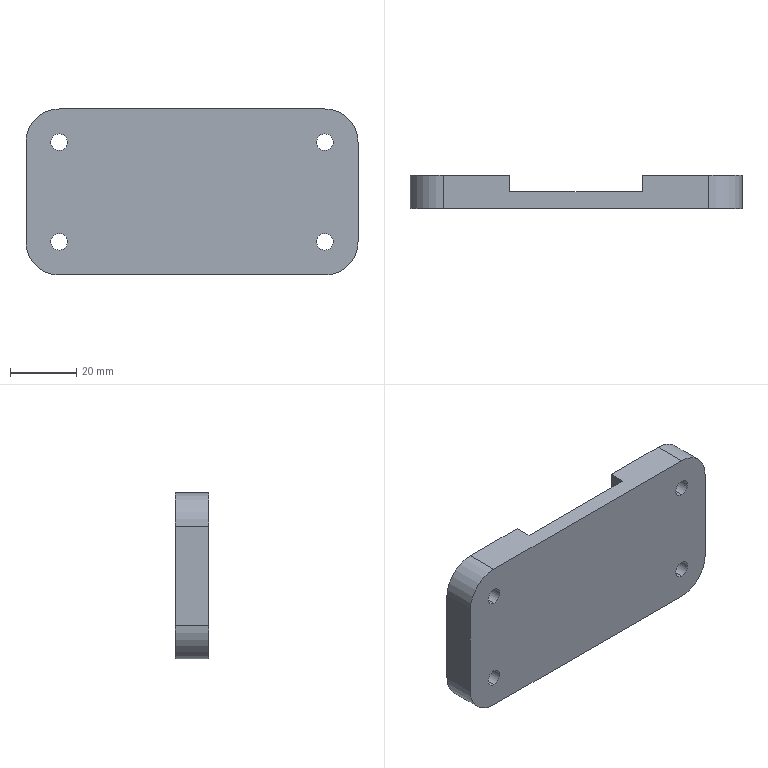Part | SolidWorks | features 3DProfileFeature 1, Extrusion 1, Fillet 1, HoleWzd 1, ICE 1 | 1 solid | 22 faces | box 100 x 10 x 50 mm | volume 38356 mm3 | cylinder 12 | plane 10 | commonest cylinder face diameters 5 x8 20 x4
STEP:
#1=CARTESIAN_POINT('',(-40.,0.,17.5));
#2=VERTEX_POINT('',#1);
#3=CARTESIAN_POINT('',(-40.,0.,12.5));
#4=VERTEX_POINT('',#3);
#5=CARTESIAN_POINT('',(-40.,0.,15.));
#6=DIRECTION('',(0.,-1.,0.));
#7=DIRECTION('',(0.,0.,-1.));
#8=AXIS2_PLACEMENT_3D('',#5,#6,#7);
#9=CIRCLE('',#8,2.5);
#10=EDGE_CURVE('',#2,#4,#9,.T.);
#11=ORIENTED_EDGE('',*,*,#10,.T.);
#12=CARTESIAN_POINT('',(-40.,10.,12.5));
#13=VERTEX_POINT('',#12);
#14=CARTESIAN_POINT('',(-40.,10.,12.5));
#15=DIRECTION('',(0.,1.,0.));
#16=VECTOR('',#15,1000.);
#17=LINE('',#14,#16);
#18=EDGE_CURVE('',#4,#13,#17,.T.);
#19=ORIENTED_EDGE('',*,*,#18,.T.);
#20=CARTESIAN_POINT('',(-40.,10.,17.5));
#21=VERTEX_POINT('',#20);
#22=CARTESIAN_POINT('',(-40.,10.,15.));
#23=DIRECTION('',(0.,1.,0.));
#24=DIRECTION('',(0.,0.,1.));
#25=AXIS2_PLACEMENT_3D('',#22,#23,#24);
#26=CIRCLE('',#25,2.5);
#27=EDGE_CURVE('',#13,#21,#26,.T.);
#28=ORIENTED_EDGE('',*,*,#27,.T.);
#29=CARTESIAN_POINT('',(-40.,10.,17.5));
#30=DIRECTION('',(0.,1.,0.));
#31=VECTOR('',#30,1000.);
#32=LINE('',#29,#31);
#33=EDGE_CURVE('',#2,#21,#32,.T.);
#34=ORIENTED_EDGE('',*,*,#33,.F.);
#35=EDGE_LOOP('',(#11,#19,#28,#34));
#36=FACE_OUTER_BOUND('',#35,.T.);
#37=CARTESIAN_POINT('',(-40.,10.,15.));
#38=DIRECTION('',(0.,1.,0.));
#39=DIRECTION('',(0.,0.,1.));
#40=AXIS2_PLACEMENT_3D('',#37,#38,#39);
#41=CYLINDRICAL_SURFACE('',#40,2.5);
#42=ADVANCED_FACE('',(#36),#41,.F.);
#43=CARTESIAN_POINT('',(-40.,0.,-12.5));
#44=VERTEX_POINT('',#43);
#45=CARTESIAN_POINT('',(-40.,0.,-17.5));
#46=VERTEX_POINT('',#45);
#47=CARTESIAN_POINT('',(-40.,0.,-15.));
#48=DIRECTION('',(0.,-1.,0.));
#49=DIRECTION('',(0.,0.,-1.));
#50=AXIS2_PLACEMENT_3D('',#47,#48,#49);
#51=CIRCLE('',#50,2.5);
#52=EDGE_CURVE('',#44,#46,#51,.T.);
#53=ORIENTED_EDGE('',*,*,#52,.T.);
#54=CARTESIAN_POINT('',(-40.,10.,-17.5));
#55=VERTEX_POINT('',#54);
#56=CARTESIAN_POINT('',(-40.,10.,-17.5));
#57=DIRECTION('',(0.,1.,0.));
#58=VECTOR('',#57,1000.);
#59=LINE('',#56,#58);
#60=EDGE_CURVE('',#46,#55,#59,.T.);
#61=ORIENTED_EDGE('',*,*,#60,.T.);
#62=CARTESIAN_POINT('',(-40.,10.,-12.5));
#63=VERTEX_POINT('',#62);
#64=CARTESIAN_POINT('',(-40.,10.,-15.));
#65=DIRECTION('',(0.,1.,0.));
#66=DIRECTION('',(0.,0.,1.));
#67=AXIS2_PLACEMENT_3D('',#64,#65,#66);
#68=CIRCLE('',#67,2.5);
#69=EDGE_CURVE('',#55,#63,#68,.T.);
#70=ORIENTED_EDGE('',*,*,#69,.T.);
#71=CARTESIAN_POINT('',(-40.,10.,-12.5));
#72=DIRECTION('',(0.,1.,0.));
#73=VECTOR('',#72,1000.);
#74=LINE('',#71,#73);
#75=EDGE_CURVE('',#44,#63,#74,.T.);
#76=ORIENTED_EDGE('',*,*,#75,.F.);
#77=EDGE_LOOP('',(#53,#61,#70,#76));
#78=FACE_OUTER_BOUND('',#77,.T.);
#79=CARTESIAN_POINT('',(-40.,10.,-15.));
#80=DIRECTION('',(0.,1.,0.));
#81=DIRECTION('',(0.,0.,1.));
#82=AXIS2_PLACEMENT_3D('',#79,#80,#81);
#83=CYLINDRICAL_SURFACE('',#82,2.5);
#84=ADVANCED_FACE('',(#78),#83,.F.);
#85=CARTESIAN_POINT('',(40.,0.,-12.5));
#86=VERTEX_POINT('',#85);
#87=CARTESIAN_POINT('',(40.,0.,-17.5));
#88=VERTEX_POINT('',#87);
#89=CARTESIAN_POINT('',(40.,0.,-15.));
#90=DIRECTION('',(0.,-1.,0.));
#91=DIRECTION('',(0.,0.,-1.));
#92=AXIS2_PLACEMENT_3D('',#89,#90,#91);
#93=CIRCLE('',#92,2.5);
#94=EDGE_CURVE('',#86,#88,#93,.T.);
#95=ORIENTED_EDGE('',*,*,#94,.T.);
#96=CARTESIAN_POINT('',(40.,10.,-17.5));
#97=VERTEX_POINT('',#96);
#98=CARTESIAN_POINT('',(40.,10.,-17.5));
#99=DIRECTION('',(0.,1.,0.));
#100=VECTOR('',#99,1000.);
#101=LINE('',#98,#100);
#102=EDGE_CURVE('',#88,#97,#101,.T.);
#103=ORIENTED_EDGE('',*,*,#102,.T.);
#104=CARTESIAN_POINT('',(40.,10.,-12.5));
#105=VERTEX_POINT('',#104);
#106=CARTESIAN_POINT('',(40.,10.,-15.));
#107=DIRECTION('',(0.,1.,0.));
#108=DIRECTION('',(0.,0.,1.));
#109=AXIS2_PLACEMENT_3D('',#106,#107,#108);
#110=CIRCLE('',#109,2.5);
#111=EDGE_CURVE('',#97,#105,#110,.T.);
#112=ORIENTED_EDGE('',*,*,#111,.T.);
#113=CARTESIAN_POINT('',(40.,10.,-12.5));
#114=DIRECTION('',(0.,1.,0.));
#115=VECTOR('',#114,1000.);
#116=LINE('',#113,#115);
#117=EDGE_CURVE('',#86,#105,#116,.T.);
#118=ORIENTED_EDGE('',*,*,#117,.F.);
#119=EDGE_LOOP('',(#95,#103,#112,#118));
#120=FACE_OUTER_BOUND('',#119,.T.);
#121=CARTESIAN_POINT('',(40.,10.,-15.));
#122=DIRECTION('',(0.,1.,0.));
#123=DIRECTION('',(0.,0.,1.));
#124=AXIS2_PLACEMENT_3D('',#121,#122,#123);
#125=CYLINDRICAL_SURFACE('',#124,2.5);
#126=ADVANCED_FACE('',(#120),#125,.F.);
#127=CARTESIAN_POINT('',(40.,0.,17.5));
#128=VERTEX_POINT('',#127);
#129=CARTESIAN_POINT('',(40.,0.,12.5));
#130=VERTEX_POINT('',#129);
#131=CARTESIAN_POINT('',(40.,0.,15.));
#132=DIRECTION('',(0.,-1.,0.));
#133=DIRECTION('',(0.,0.,-1.));
#134=AXIS2_PLACEMENT_3D('',#131,#132,#133);
#135=CIRCLE('',#134,2.5);
#136=EDGE_CURVE('',#128,#130,#135,.T.);
#137=ORIENTED_EDGE('',*,*,#136,.T.);
#138=CARTESIAN_POINT('',(40.,10.,12.5));
#139=VERTEX_POINT('',#138);
#140=CARTESIAN_POINT('',(40.,10.,12.5));
#141=DIRECTION('',(0.,1.,0.));
#142=VECTOR('',#141,1000.);
#143=LINE('',#140,#142);
#144=EDGE_CURVE('',#130,#139,#143,.T.);
#145=ORIENTED_EDGE('',*,*,#144,.T.);
#146=CARTESIAN_POINT('',(40.,10.,17.5));
#147=VERTEX_POINT('',#146);
#148=CARTESIAN_POINT('',(40.,10.,15.));
#149=DIRECTION('',(0.,1.,0.));
#150=DIRECTION('',(0.,0.,1.));
#151=AXIS2_PLACEMENT_3D('',#148,#149,#150);
#152=CIRCLE('',#151,2.5);
#153=EDGE_CURVE('',#139,#147,#152,.T.);
#154=ORIENTED_EDGE('',*,*,#153,.T.);
#155=CARTESIAN_POINT('',(40.,10.,17.5));
#156=DIRECTION('',(0.,1.,0.));
#157=VECTOR('',#156,1000.);
#158=LINE('',#155,#157);
#159=EDGE_CURVE('',#128,#147,#158,.T.);
#160=ORIENTED_EDGE('',*,*,#159,.F.);
#161=EDGE_LOOP('',(#137,#145,#154,#160));
#162=FACE_OUTER_BOUND('',#161,.T.);
#163=CARTESIAN_POINT('',(40.,10.,15.));
#164=DIRECTION('',(0.,1.,0.));
#165=DIRECTION('',(0.,0.,1.));
#166=AXIS2_PLACEMENT_3D('',#163,#164,#165);
#167=CYLINDRICAL_SURFACE('',#166,2.5);
#168=ADVANCED_FACE('',(#162),#167,.F.);
#169=CARTESIAN_POINT('',(40.,10.,15.));
#170=DIRECTION('',(0.,1.,0.));
#171=DIRECTION('',(0.,0.,1.));
#172=AXIS2_PLACEMENT_3D('',#169,#170,#171);
#173=CIRCLE('',#172,2.5);
#174=EDGE_CURVE('',#147,#139,#173,.T.);
#175=ORIENTED_EDGE('',*,*,#174,.F.);
#176=ORIENTED_EDGE('',*,*,#153,.F.);
#177=EDGE_LOOP('',(#175,#176));
#178=FACE_BOUND('',#177,.T.);
#179=CARTESIAN_POINT('',(40.,10.,-15.));
#180=DIRECTION('',(0.,1.,0.));
#181=DIRECTION('',(0.,0.,1.));
#182=AXIS2_PLACEMENT_3D('',#179,#180,#181);
#183=CIRCLE('',#182,2.5);
#184=EDGE_CURVE('',#105,#97,#183,.T.);
#185=ORIENTED_EDGE('',*,*,#184,.F.);
#186=ORIENTED_EDGE('',*,*,#111,.F.);
#187=EDGE_LOOP('',(#185,#186));
#188=FACE_BOUND('',#187,.T.);
#189=CARTESIAN_POINT('',(40.,10.,-25.));
#190=VERTEX_POINT('',#189);
#191=CARTESIAN_POINT('',(20.,10.,-25.));
#192=VERTEX_POINT('',#191);
#193=CARTESIAN_POINT('',(-50.,10.,-25.));
#194=DIRECTION('',(-1.,0.,0.));
#195=VECTOR('',#194,1000.);
#196=LINE('',#193,#195);
#197=EDGE_CURVE('',#190,#192,#196,.T.);
#198=ORIENTED_EDGE('',*,*,#197,.T.);
#199=CARTESIAN_POINT('',(20.,10.,25.));
#200=VERTEX_POINT('',#199);
#201=CARTESIAN_POINT('',(20.,10.,25.));
#202=DIRECTION('',(0.,0.,-1.));
#203=VECTOR('',#202,1000.);
#204=LINE('',#201,#203);
#205=EDGE_CURVE('',#200,#192,#204,.T.);
#206=ORIENTED_EDGE('',*,*,#205,.F.);
#207=CARTESIAN_POINT('',(40.,10.,25.));
#208=VERTEX_POINT('',#207);
#209=CARTESIAN_POINT('',(-50.,10.,25.));
#210=DIRECTION('',(1.,0.,0.));
#211=VECTOR('',#210,1000.);
#212=LINE('',#209,#211);
#213=EDGE_CURVE('',#200,#208,#212,.T.);
#214=ORIENTED_EDGE('',*,*,#213,.T.);
#215=CARTESIAN_POINT('',(50.,10.,15.));
#216=VERTEX_POINT('',#215);
#217=CARTESIAN_POINT('',(40.,10.,15.));
#218=DIRECTION('',(0.,1.,0.));
#219=DIRECTION('',(0.,0.,-1.));
#220=AXIS2_PLACEMENT_3D('',#217,#218,#219);
#221=CIRCLE('',#220,10.);
#222=EDGE_CURVE('',#208,#216,#221,.T.);
#223=ORIENTED_EDGE('',*,*,#222,.T.);
#224=CARTESIAN_POINT('',(50.,10.,-15.));
#225=VERTEX_POINT('',#224);
#226=CARTESIAN_POINT('',(50.,10.,25.));
#227=DIRECTION('',(0.,0.,-1.));
#228=VECTOR('',#227,1000.);
#229=LINE('',#226,#228);
#230=EDGE_CURVE('',#216,#225,#229,.T.);
#231=ORIENTED_EDGE('',*,*,#230,.T.);
#232=CARTESIAN_POINT('',(40.,10.,-15.));
#233=DIRECTION('',(0.,1.,0.));
#234=DIRECTION('',(0.,0.,-1.));
#235=AXIS2_PLACEMENT_3D('',#232,#233,#234);
#236=CIRCLE('',#235,10.);
#237=EDGE_CURVE('',#225,#190,#236,.T.);
#238=ORIENTED_EDGE('',*,*,#237,.T.);
#239=EDGE_LOOP('',(#198,#206,#214,#223,#231,#238));
#240=FACE_OUTER_BOUND('',#239,.T.);
#241=CARTESIAN_POINT('',(0.,10.,0.));
#242=DIRECTION('',(0.,-1.,0.));
#243=DIRECTION('',(0.,0.,-1.));
#244=AXIS2_PLACEMENT_3D('',#241,#242,#243);
#245=PLANE('',#244);
#246=ADVANCED_FACE('',(#178,#188,#240),#245,.F.);
#247=CARTESIAN_POINT('',(50.,0.,15.));
#248=VERTEX_POINT('',#247);
#249=CARTESIAN_POINT('',(50.,0.,-15.));
#250=VERTEX_POINT('',#249);
#251=CARTESIAN_POINT('',(50.,0.,25.));
#252=DIRECTION('',(0.,0.,-1.));
#253=VECTOR('',#252,1000.);
#254=LINE('',#251,#253);
#255=EDGE_CURVE('',#248,#250,#254,.T.);
#256=ORIENTED_EDGE('',*,*,#255,.T.);
#257=CARTESIAN_POINT('',(50.,10.,-15.));
#258=DIRECTION('',(0.,1.,0.));
#259=VECTOR('',#258,1000.);
#260=LINE('',#257,#259);
#261=EDGE_CURVE('',#250,#225,#260,.T.);
#262=ORIENTED_EDGE('',*,*,#261,.T.);
#263=ORIENTED_EDGE('',*,*,#230,.F.);
#264=CARTESIAN_POINT('',(50.,10.,15.));
#265=DIRECTION('',(0.,-1.,0.));
#266=VECTOR('',#265,1000.);
#267=LINE('',#264,#266);
#268=EDGE_CURVE('',#216,#248,#267,.T.);
#269=ORIENTED_EDGE('',*,*,#268,.T.);
#270=EDGE_LOOP('',(#256,#262,#263,#269));
#271=FACE_OUTER_BOUND('',#270,.T.);
#272=CARTESIAN_POINT('',(50.,10.,25.));
#273=DIRECTION('',(-1.,0.,0.));
#274=DIRECTION('',(0.,0.,1.));
#275=AXIS2_PLACEMENT_3D('',#272,#273,#274);
#276=PLANE('',#275);
#277=ADVANCED_FACE('',(#271),#276,.F.);
#278=CARTESIAN_POINT('',(20.,5.,-25.));
#279=VERTEX_POINT('',#278);
#280=CARTESIAN_POINT('',(-20.,5.,-25.));
#281=VERTEX_POINT('',#280);
#282=CARTESIAN_POINT('',(-20.,5.,-25.));
#283=DIRECTION('',(-1.,0.,0.));
#284=VECTOR('',#283,1000.);
#285=LINE('',#282,#284);
#286=EDGE_CURVE('',#279,#281,#285,.T.);
#287=ORIENTED_EDGE('',*,*,#286,.F.);
#288=CARTESIAN_POINT('',(20.,5.,-25.));
#289=DIRECTION('',(0.,1.,0.));
#290=VECTOR('',#289,1000.);
#291=LINE('',#288,#290);
#292=EDGE_CURVE('',#279,#192,#291,.T.);
#293=ORIENTED_EDGE('',*,*,#292,.T.);
#294=ORIENTED_EDGE('',*,*,#197,.F.);
#295=CARTESIAN_POINT('',(40.,0.,-25.));
#296=VERTEX_POINT('',#295);
#297=CARTESIAN_POINT('',(40.,10.,-25.));
#298=DIRECTION('',(0.,-1.,0.));
#299=VECTOR('',#298,1000.);
#300=LINE('',#297,#299);
#301=EDGE_CURVE('',#190,#296,#300,.T.);
#302=ORIENTED_EDGE('',*,*,#301,.T.);
#303=CARTESIAN_POINT('',(-40.,0.,-25.));
#304=VERTEX_POINT('',#303);
#305=CARTESIAN_POINT('',(-50.,0.,-25.));
#306=DIRECTION('',(-1.,0.,0.));
#307=VECTOR('',#306,1000.);
#308=LINE('',#305,#307);
#309=EDGE_CURVE('',#296,#304,#308,.T.);
#310=ORIENTED_EDGE('',*,*,#309,.T.);
#311=CARTESIAN_POINT('',(-40.,10.,-25.));
#312=VERTEX_POINT('',#311);
#313=CARTESIAN_POINT('',(-40.,10.,-25.));
#314=DIRECTION('',(0.,1.,0.));
#315=VECTOR('',#314,1000.);
#316=LINE('',#313,#315);
#317=EDGE_CURVE('',#304,#312,#316,.T.);
#318=ORIENTED_EDGE('',*,*,#317,.T.);
#319=CARTESIAN_POINT('',(-20.,10.,-25.));
#320=VERTEX_POINT('',#319);
#321=CARTESIAN_POINT('',(-50.,10.,-25.));
#322=DIRECTION('',(-1.,0.,0.));
#323=VECTOR('',#322,1000.);
#324=LINE('',#321,#323);
#325=EDGE_CURVE('',#320,#312,#324,.T.);
#326=ORIENTED_EDGE('',*,*,#325,.F.);
#327=CARTESIAN_POINT('',(-20.,5.,-25.));
#328=DIRECTION('',(0.,1.,0.));
#329=VECTOR('',#328,1000.);
#330=LINE('',#327,#329);
#331=EDGE_CURVE('',#281,#320,#330,.T.);
#332=ORIENTED_EDGE('',*,*,#331,.F.);
#333=EDGE_LOOP('',(#287,#293,#294,#302,#310,#318,#326,#332));
#334=FACE_OUTER_BOUND('',#333,.T.);
#335=CARTESIAN_POINT('',(-50.,10.,-25.));
#336=DIRECTION('',(0.,0.,1.));
#337=DIRECTION('',(1.,0.,0.));
#338=AXIS2_PLACEMENT_3D('',#335,#336,#337);
#339=PLANE('',#338);
#340=ADVANCED_FACE('',(#334),#339,.F.);
#341=CARTESIAN_POINT('',(-50.,10.,-15.));
#342=VERTEX_POINT('',#341);
#343=CARTESIAN_POINT('',(-50.,10.,15.));
#344=VERTEX_POINT('',#343);
#345=CARTESIAN_POINT('',(-50.,10.,25.));
#346=DIRECTION('',(0.,0.,1.));
#347=VECTOR('',#346,1000.);
#348=LINE('',#345,#347);
#349=EDGE_CURVE('',#342,#344,#348,.T.);
#350=ORIENTED_EDGE('',*,*,#349,.F.);
#351=CARTESIAN_POINT('',(-50.,0.,-15.));
#352=VERTEX_POINT('',#351);
#353=CARTESIAN_POINT('',(-50.,10.,-15.));
#354=DIRECTION('',(0.,-1.,0.));
#355=VECTOR('',#354,1000.);
#356=LINE('',#353,#355);
#357=EDGE_CURVE('',#342,#352,#356,.T.);
#358=ORIENTED_EDGE('',*,*,#357,.T.);
#359=CARTESIAN_POINT('',(-50.,0.,15.));
#360=VERTEX_POINT('',#359);
#361=CARTESIAN_POINT('',(-50.,0.,25.));
#362=DIRECTION('',(0.,0.,1.));
#363=VECTOR('',#362,1000.);
#364=LINE('',#361,#363);
#365=EDGE_CURVE('',#352,#360,#364,.T.);
#366=ORIENTED_EDGE('',*,*,#365,.T.);
#367=CARTESIAN_POINT('',(-50.,10.,15.));
#368=DIRECTION('',(0.,1.,0.));
#369=VECTOR('',#368,1000.);
#370=LINE('',#367,#369);
#371=EDGE_CURVE('',#360,#344,#370,.T.);
#372=ORIENTED_EDGE('',*,*,#371,.T.);
#373=EDGE_LOOP('',(#350,#358,#366,#372));
#374=FACE_OUTER_BOUND('',#373,.T.);
#375=CARTESIAN_POINT('',(-50.,10.,25.));
#376=DIRECTION('',(1.,0.,0.));
#377=DIRECTION('',(0.,0.,-1.));
#378=AXIS2_PLACEMENT_3D('',#375,#376,#377);
#379=PLANE('',#378);
#380=ADVANCED_FACE('',(#374),#379,.F.);
#381=ORIENTED_EDGE('',*,*,#213,.F.);
#382=CARTESIAN_POINT('',(20.,5.,25.));
#383=VERTEX_POINT('',#382);
#384=CARTESIAN_POINT('',(20.,5.,25.));
#385=DIRECTION('',(0.,1.,0.));
#386=VECTOR('',#385,1000.);
#387=LINE('',#384,#386);
#388=EDGE_CURVE('',#383,#200,#387,.T.);
#389=ORIENTED_EDGE('',*,*,#388,.F.);
#390=CARTESIAN_POINT('',(-20.,5.,25.));
#391=VERTEX_POINT('',#390);
#392=CARTESIAN_POINT('',(-20.,5.,25.));
#393=DIRECTION('',(1.,0.,0.));
#394=VECTOR('',#393,1000.);
#395=LINE('',#392,#394);
#396=EDGE_CURVE('',#391,#383,#395,.T.);
#397=ORIENTED_EDGE('',*,*,#396,.F.);
#398=CARTESIAN_POINT('',(-20.,10.,25.));
#399=VERTEX_POINT('',#398);
#400=CARTESIAN_POINT('',(-20.,5.,25.));
#401=DIRECTION('',(0.,1.,0.));
#402=VECTOR('',#401,1000.);
#403=LINE('',#400,#402);
#404=EDGE_CURVE('',#391,#399,#403,.T.);
#405=ORIENTED_EDGE('',*,*,#404,.T.);
#406=CARTESIAN_POINT('',(-40.,10.,25.));
#407=VERTEX_POINT('',#406);
#408=CARTESIAN_POINT('',(-50.,10.,25.));
#409=DIRECTION('',(1.,0.,0.));
#410=VECTOR('',#409,1000.);
#411=LINE('',#408,#410);
#412=EDGE_CURVE('',#407,#399,#411,.T.);
#413=ORIENTED_EDGE('',*,*,#412,.F.);
#414=CARTESIAN_POINT('',(-40.,0.,25.));
#415=VERTEX_POINT('',#414);
#416=CARTESIAN_POINT('',(-40.,10.,25.));
#417=DIRECTION('',(0.,-1.,0.));
#418=VECTOR('',#417,1000.);
#419=LINE('',#416,#418);
#420=EDGE_CURVE('',#407,#415,#419,.T.);
#421=ORIENTED_EDGE('',*,*,#420,.T.);
#422=CARTESIAN_POINT('',(40.,0.,25.));
#423=VERTEX_POINT('',#422);
#424=CARTESIAN_POINT('',(-50.,0.,25.));
#425=DIRECTION('',(1.,0.,0.));
#426=VECTOR('',#425,1000.);
#427=LINE('',#424,#426);
#428=EDGE_CURVE('',#415,#423,#427,.T.);
#429=ORIENTED_EDGE('',*,*,#428,.T.);
#430=CARTESIAN_POINT('',(40.,10.,25.));
#431=DIRECTION('',(0.,1.,0.));
#432=VECTOR('',#431,1000.);
#433=LINE('',#430,#432);
#434=EDGE_CURVE('',#423,#208,#433,.T.);
#435=ORIENTED_EDGE('',*,*,#434,.T.);
#436=EDGE_LOOP('',(#381,#389,#397,#405,#413,#421,#429,#435));
#437=FACE_OUTER_BOUND('',#436,.T.);
#438=CARTESIAN_POINT('',(-50.,10.,25.));
#439=DIRECTION('',(0.,0.,-1.));
#440=DIRECTION('',(-1.,0.,0.));
#441=AXIS2_PLACEMENT_3D('',#438,#439,#440);
#442=PLANE('',#441);
#443=ADVANCED_FACE('',(#437),#442,.F.);
#444=CARTESIAN_POINT('',(-40.,10.,15.));
#445=DIRECTION('',(0.,1.,0.));
#446=DIRECTION('',(0.,0.,1.));
#447=AXIS2_PLACEMENT_3D('',#444,#445,#446);
#448=CIRCLE('',#447,2.5);
#449=EDGE_CURVE('',#21,#13,#448,.T.);
#450=ORIENTED_EDGE('',*,*,#449,.F.);
#451=ORIENTED_EDGE('',*,*,#27,.F.);
#452=EDGE_LOOP('',(#450,#451));
#453=FACE_BOUND('',#452,.T.);
#454=CARTESIAN_POINT('',(-40.,10.,-15.));
#455=DIRECTION('',(0.,1.,0.));
#456=DIRECTION('',(0.,0.,1.));
#457=AXIS2_PLACEMENT_3D('',#454,#455,#456);
#458=CIRCLE('',#457,2.5);
#459=EDGE_CURVE('',#63,#55,#458,.T.);
#460=ORIENTED_EDGE('',*,*,#459,.F.);
#461=ORIENTED_EDGE('',*,*,#69,.F.);
#462=EDGE_LOOP('',(#460,#461));
#463=FACE_BOUND('',#462,.T.);
#464=ORIENTED_EDGE('',*,*,#412,.T.);
#465=CARTESIAN_POINT('',(-20.,10.,25.));
#466=DIRECTION('',(0.,0.,1.));
#467=VECTOR('',#466,1000.);
#468=LINE('',#465,#467);
#469=EDGE_CURVE('',#320,#399,#468,.T.);
#470=ORIENTED_EDGE('',*,*,#469,.F.);
#471=ORIENTED_EDGE('',*,*,#325,.T.);
#472=CARTESIAN_POINT('',(-40.,10.,-15.));
#473=DIRECTION('',(0.,1.,0.));
#474=DIRECTION('',(0.,0.,-1.));
#475=AXIS2_PLACEMENT_3D('',#472,#473,#474);
#476=CIRCLE('',#475,10.);
#477=EDGE_CURVE('',#312,#342,#476,.T.);
#478=ORIENTED_EDGE('',*,*,#477,.T.);
#479=ORIENTED_EDGE('',*,*,#349,.T.);
#480=CARTESIAN_POINT('',(-40.,10.,15.));
#481=DIRECTION('',(0.,1.,0.));
#482=DIRECTION('',(0.,0.,-1.));
#483=AXIS2_PLACEMENT_3D('',#480,#481,#482);
#484=CIRCLE('',#483,10.);
#485=EDGE_CURVE('',#344,#407,#484,.T.);
#486=ORIENTED_EDGE('',*,*,#485,.T.);
#487=EDGE_LOOP('',(#464,#470,#471,#478,#479,#486));
#488=FACE_OUTER_BOUND('',#487,.T.);
#489=CARTESIAN_POINT('',(0.,10.,0.));
#490=DIRECTION('',(0.,-1.,0.));
#491=DIRECTION('',(0.,0.,-1.));
#492=AXIS2_PLACEMENT_3D('',#489,#490,#491);
#493=PLANE('',#492);
#494=ADVANCED_FACE('',(#453,#463,#488),#493,.F.);
#495=ORIENTED_EDGE('',*,*,#10,.F.);
#496=CARTESIAN_POINT('',(-40.,0.,15.));
#497=DIRECTION('',(0.,-1.,0.));
#498=DIRECTION('',(0.,0.,-1.));
#499=AXIS2_PLACEMENT_3D('',#496,#497,#498);
#500=CIRCLE('',#499,2.5);
#501=EDGE_CURVE('',#4,#2,#500,.T.);
#502=ORIENTED_EDGE('',*,*,#501,.F.);
#503=EDGE_LOOP('',(#495,#502));
#504=FACE_BOUND('',#503,.T.);
#505=ORIENTED_EDGE('',*,*,#52,.F.);
#506=CARTESIAN_POINT('',(-40.,0.,-15.));
#507=DIRECTION('',(0.,-1.,0.));
#508=DIRECTION('',(0.,0.,-1.));
#509=AXIS2_PLACEMENT_3D('',#506,#507,#508);
#510=CIRCLE('',#509,2.5);
#511=EDGE_CURVE('',#46,#44,#510,.T.);
#512=ORIENTED_EDGE('',*,*,#511,.F.);
#513=EDGE_LOOP('',(#505,#512));
#514=FACE_BOUND('',#513,.T.);
#515=ORIENTED_EDGE('',*,*,#94,.F.);
#516=CARTESIAN_POINT('',(40.,0.,-15.));
#517=DIRECTION('',(0.,-1.,0.));
#518=DIRECTION('',(0.,0.,-1.));
#519=AXIS2_PLACEMENT_3D('',#516,#517,#518);
#520=CIRCLE('',#519,2.5);
#521=EDGE_CURVE('',#88,#86,#520,.T.);
#522=ORIENTED_EDGE('',*,*,#521,.F.);
#523=EDGE_LOOP('',(#515,#522));
#524=FACE_BOUND('',#523,.T.);
#525=ORIENTED_EDGE('',*,*,#136,.F.);
#526=CARTESIAN_POINT('',(40.,0.,15.));
#527=DIRECTION('',(0.,-1.,0.));
#528=DIRECTION('',(0.,0.,-1.));
#529=AXIS2_PLACEMENT_3D('',#526,#527,#528);
#530=CIRCLE('',#529,2.5);
#531=EDGE_CURVE('',#130,#128,#530,.T.);
#532=ORIENTED_EDGE('',*,*,#531,.F.);
#533=EDGE_LOOP('',(#525,#532));
#534=FACE_BOUND('',#533,.T.);
#535=ORIENTED_EDGE('',*,*,#365,.F.);
#536=CARTESIAN_POINT('',(-40.,0.,-15.));
#537=DIRECTION('',(0.,-1.,0.));
#538=DIRECTION('',(0.,0.,-1.));
#539=AXIS2_PLACEMENT_3D('',#536,#537,#538);
#540=CIRCLE('',#539,10.);
#541=EDGE_CURVE('',#352,#304,#540,.T.);
#542=ORIENTED_EDGE('',*,*,#541,.T.);
#543=ORIENTED_EDGE('',*,*,#309,.F.);
#544=CARTESIAN_POINT('',(40.,0.,-15.));
#545=DIRECTION('',(0.,-1.,0.));
#546=DIRECTION('',(0.,0.,-1.));
#547=AXIS2_PLACEMENT_3D('',#544,#545,#546);
#548=CIRCLE('',#547,10.);
#549=EDGE_CURVE('',#296,#250,#548,.T.);
#550=ORIENTED_EDGE('',*,*,#549,.T.);
#551=ORIENTED_EDGE('',*,*,#255,.F.);
#552=CARTESIAN_POINT('',(40.,0.,15.));
#553=DIRECTION('',(0.,-1.,0.));
#554=DIRECTION('',(0.,0.,-1.));
#555=AXIS2_PLACEMENT_3D('',#552,#553,#554);
#556=CIRCLE('',#555,10.);
#557=EDGE_CURVE('',#248,#423,#556,.T.);
#558=ORIENTED_EDGE('',*,*,#557,.T.);
#559=ORIENTED_EDGE('',*,*,#428,.F.);
#560=CARTESIAN_POINT('',(-40.,0.,15.));
#561=DIRECTION('',(0.,-1.,0.));
#562=DIRECTION('',(0.,0.,-1.));
#563=AXIS2_PLACEMENT_3D('',#560,#561,#562);
#564=CIRCLE('',#563,10.);
#565=EDGE_CURVE('',#415,#360,#564,.T.);
#566=ORIENTED_EDGE('',*,*,#565,.T.);
#567=EDGE_LOOP('',(#535,#542,#543,#550,#551,#558,#559,#566));
#568=FACE_OUTER_BOUND('',#567,.T.);
#569=CARTESIAN_POINT('',(0.,0.,0.));
#570=DIRECTION('',(0.,-1.,0.));
#571=DIRECTION('',(0.,0.,-1.));
#572=AXIS2_PLACEMENT_3D('',#569,#570,#571);
#573=PLANE('',#572);
#574=ADVANCED_FACE('',(#504,#514,#524,#534,#568),#573,.T.);
#575=ORIENTED_EDGE('',*,*,#477,.F.);
#576=ORIENTED_EDGE('',*,*,#317,.F.);
#577=ORIENTED_EDGE('',*,*,#541,.F.);
#578=ORIENTED_EDGE('',*,*,#357,.F.);
#579=EDGE_LOOP('',(#575,#576,#577,#578));
#580=FACE_OUTER_BOUND('',#579,.T.);
#581=CARTESIAN_POINT('',(-40.,10.,-15.));
#582=DIRECTION('',(0.,-1.,0.));
#583=DIRECTION('',(0.,0.,-1.));
#584=AXIS2_PLACEMENT_3D('',#581,#582,#583);
#585=CYLINDRICAL_SURFACE('',#584,10.);
#586=ADVANCED_FACE('',(#580),#585,.T.);
#587=ORIENTED_EDGE('',*,*,#485,.F.);
#588=ORIENTED_EDGE('',*,*,#371,.F.);
#589=ORIENTED_EDGE('',*,*,#565,.F.);
#590=ORIENTED_EDGE('',*,*,#420,.F.);
#591=EDGE_LOOP('',(#587,#588,#589,#590));
#592=FACE_OUTER_BOUND('',#591,.T.);
#593=CARTESIAN_POINT('',(-40.,10.,15.));
#594=DIRECTION('',(0.,-1.,0.));
#595=DIRECTION('',(0.,0.,-1.));
#596=AXIS2_PLACEMENT_3D('',#593,#594,#595);
#597=CYLINDRICAL_SURFACE('',#596,10.);
#598=ADVANCED_FACE('',(#592),#597,.T.);
#599=ORIENTED_EDGE('',*,*,#237,.F.);
#600=ORIENTED_EDGE('',*,*,#261,.F.);
#601=ORIENTED_EDGE('',*,*,#549,.F.);
#602=ORIENTED_EDGE('',*,*,#301,.F.);
#603=EDGE_LOOP('',(#599,#600,#601,#602));
#604=FACE_OUTER_BOUND('',#603,.T.);
#605=CARTESIAN_POINT('',(40.,10.,-15.));
#606=DIRECTION('',(0.,-1.,0.));
#607=DIRECTION('',(0.,0.,-1.));
#608=AXIS2_PLACEMENT_3D('',#605,#606,#607);
#609=CYLINDRICAL_SURFACE('',#608,10.);
#610=ADVANCED_FACE('',(#604),#609,.T.);
#611=ORIENTED_EDGE('',*,*,#222,.F.);
#612=ORIENTED_EDGE('',*,*,#434,.F.);
#613=ORIENTED_EDGE('',*,*,#557,.F.);
#614=ORIENTED_EDGE('',*,*,#268,.F.);
#615=EDGE_LOOP('',(#611,#612,#613,#614));
#616=FACE_OUTER_BOUND('',#615,.T.);
#617=CARTESIAN_POINT('',(40.,10.,15.));
#618=DIRECTION('',(0.,-1.,0.));
#619=DIRECTION('',(0.,0.,-1.));
#620=AXIS2_PLACEMENT_3D('',#617,#618,#619);
#621=CYLINDRICAL_SURFACE('',#620,10.);
#622=ADVANCED_FACE('',(#616),#621,.T.);
#623=ORIENTED_EDGE('',*,*,#144,.F.);
#624=ORIENTED_EDGE('',*,*,#531,.T.);
#625=ORIENTED_EDGE('',*,*,#159,.T.);
#626=ORIENTED_EDGE('',*,*,#174,.T.);
#627=EDGE_LOOP('',(#623,#624,#625,#626));
#628=FACE_OUTER_BOUND('',#627,.T.);
#629=CARTESIAN_POINT('',(40.,10.,15.));
#630=DIRECTION('',(0.,1.,0.));
#631=DIRECTION('',(0.,0.,1.));
#632=AXIS2_PLACEMENT_3D('',#629,#630,#631);
#633=CYLINDRICAL_SURFACE('',#632,2.5);
#634=ADVANCED_FACE('',(#628),#633,.F.);
#635=ORIENTED_EDGE('',*,*,#102,.F.);
#636=ORIENTED_EDGE('',*,*,#521,.T.);
#637=ORIENTED_EDGE('',*,*,#117,.T.);
#638=ORIENTED_EDGE('',*,*,#184,.T.);
#639=EDGE_LOOP('',(#635,#636,#637,#638));
#640=FACE_OUTER_BOUND('',#639,.T.);
#641=CARTESIAN_POINT('',(40.,10.,-15.));
#642=DIRECTION('',(0.,1.,0.));
#643=DIRECTION('',(0.,0.,1.));
#644=AXIS2_PLACEMENT_3D('',#641,#642,#643);
#645=CYLINDRICAL_SURFACE('',#644,2.5);
#646=ADVANCED_FACE('',(#640),#645,.F.);
#647=ORIENTED_EDGE('',*,*,#60,.F.);
#648=ORIENTED_EDGE('',*,*,#511,.T.);
#649=ORIENTED_EDGE('',*,*,#75,.T.);
#650=ORIENTED_EDGE('',*,*,#459,.T.);
#651=EDGE_LOOP('',(#647,#648,#649,#650));
#652=FACE_OUTER_BOUND('',#651,.T.);
#653=CARTESIAN_POINT('',(-40.,10.,-15.));
#654=DIRECTION('',(0.,1.,0.));
#655=DIRECTION('',(0.,0.,1.));
#656=AXIS2_PLACEMENT_3D('',#653,#654,#655);
#657=CYLINDRICAL_SURFACE('',#656,2.5);
#658=ADVANCED_FACE('',(#652),#657,.F.);
#659=ORIENTED_EDGE('',*,*,#18,.F.);
#660=ORIENTED_EDGE('',*,*,#501,.T.);
#661=ORIENTED_EDGE('',*,*,#33,.T.);
#662=ORIENTED_EDGE('',*,*,#449,.T.);
#663=EDGE_LOOP('',(#659,#660,#661,#662));
#664=FACE_OUTER_BOUND('',#663,.T.);
#665=CARTESIAN_POINT('',(-40.,10.,15.));
#666=DIRECTION('',(0.,1.,0.));
#667=DIRECTION('',(0.,0.,1.));
#668=AXIS2_PLACEMENT_3D('',#665,#666,#667);
#669=CYLINDRICAL_SURFACE('',#668,2.5);
#670=ADVANCED_FACE('',(#664),#669,.F.);
#671=ORIENTED_EDGE('',*,*,#205,.T.);
#672=ORIENTED_EDGE('',*,*,#292,.F.);
#673=CARTESIAN_POINT('',(20.,5.,25.));
#674=DIRECTION('',(0.,0.,-1.));
#675=VECTOR('',#674,1000.);
#676=LINE('',#673,#675);
#677=EDGE_CURVE('',#383,#279,#676,.T.);
#678=ORIENTED_EDGE('',*,*,#677,.F.);
#679=ORIENTED_EDGE('',*,*,#388,.T.);
#680=EDGE_LOOP('',(#671,#672,#678,#679));
#681=FACE_OUTER_BOUND('',#680,.T.);
#682=CARTESIAN_POINT('',(20.,5.,25.));
#683=DIRECTION('',(1.,0.,0.));
#684=DIRECTION('',(0.,0.,-1.));
#685=AXIS2_PLACEMENT_3D('',#682,#683,#684);
#686=PLANE('',#685);
#687=ADVANCED_FACE('',(#681),#686,.F.);
#688=ORIENTED_EDGE('',*,*,#469,.T.);
#689=ORIENTED_EDGE('',*,*,#404,.F.);
#690=CARTESIAN_POINT('',(-20.,5.,25.));
#691=DIRECTION('',(0.,0.,1.));
#692=VECTOR('',#691,1000.);
#693=LINE('',#690,#692);
#694=EDGE_CURVE('',#281,#391,#693,.T.);
#695=ORIENTED_EDGE('',*,*,#694,.F.);
#696=ORIENTED_EDGE('',*,*,#331,.T.);
#697=EDGE_LOOP('',(#688,#689,#695,#696));
#698=FACE_OUTER_BOUND('',#697,.T.);
#699=CARTESIAN_POINT('',(-20.,5.,25.));
#700=DIRECTION('',(-1.,0.,0.));
#701=DIRECTION('',(0.,0.,1.));
#702=AXIS2_PLACEMENT_3D('',#699,#700,#701);
#703=PLANE('',#702);
#704=ADVANCED_FACE('',(#698),#703,.F.);
#705=ORIENTED_EDGE('',*,*,#677,.T.);
#706=ORIENTED_EDGE('',*,*,#286,.T.);
#707=ORIENTED_EDGE('',*,*,#694,.T.);
#708=ORIENTED_EDGE('',*,*,#396,.T.);
#709=EDGE_LOOP('',(#705,#706,#707,#708));
#710=FACE_OUTER_BOUND('',#709,.T.);
#711=CARTESIAN_POINT('',(0.,5.,0.));
#712=DIRECTION('',(0.,-1.,0.));
#713=DIRECTION('',(0.,0.,-1.));
#714=AXIS2_PLACEMENT_3D('',#711,#712,#713);
#715=PLANE('',#714);
#716=ADVANCED_FACE('',(#710),#715,.F.);
#717=CLOSED_SHELL('',(#42,#84,#126,#168,#246,#277,#340,#380,#443,#494,#574,#586,#598,#610,#622,#634,#646,#658,#670,#687,#704,#716));
#718=MANIFOLD_SOLID_BREP('',#717);
#719=CARTESIAN_POINT('',(0.,0.,0.));
#720=DIRECTION('',(0.,0.,1.));
#721=DIRECTION('',(1.,0.,0.));
#722=AXIS2_PLACEMENT_3D('',#719,#720,#721);
#723=(LENGTH_UNIT()NAMED_UNIT(*)SI_UNIT(.MILLI.,.METRE.));
#724=UNCERTAINTY_MEASURE_WITH_UNIT(LENGTH_MEASURE(0.00001),#723,'','');
#725=(NAMED_UNIT(*)PLANE_ANGLE_UNIT()SI_UNIT($,.RADIAN.));
#726=(NAMED_UNIT(*)SI_UNIT($,.STERADIAN.)SOLID_ANGLE_UNIT());
#727=(GEOMETRIC_REPRESENTATION_CONTEXT(3)GLOBAL_UNCERTAINTY_ASSIGNED_CONTEXT((#724))GLOBAL_UNIT_ASSIGNED_CONTEXT((#723,#725,#726))REPRESENTATION_CONTEXT('',''));
#728=ADVANCED_BREP_SHAPE_REPRESENTATION('',(#718,#722),#727);